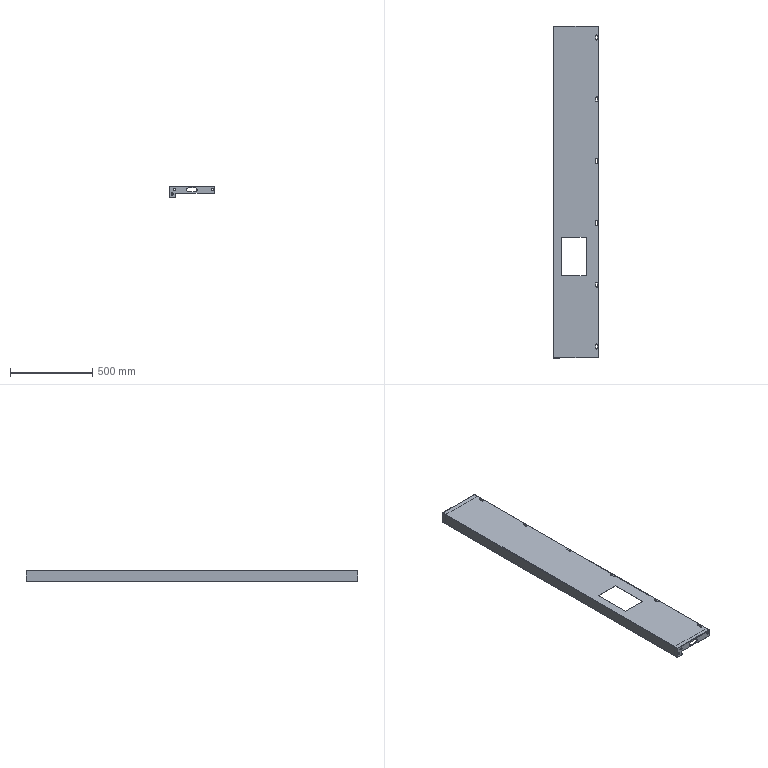Part | 3 solids | 220 faces | box 275 x 2016 x 70 mm | volume 1089729 mm3 | plane 134 | cylinder 86 | commonest cylinder face diameters 6.2 x28 9 x18 11 x10 3.4 x9 10 x6 24 x6